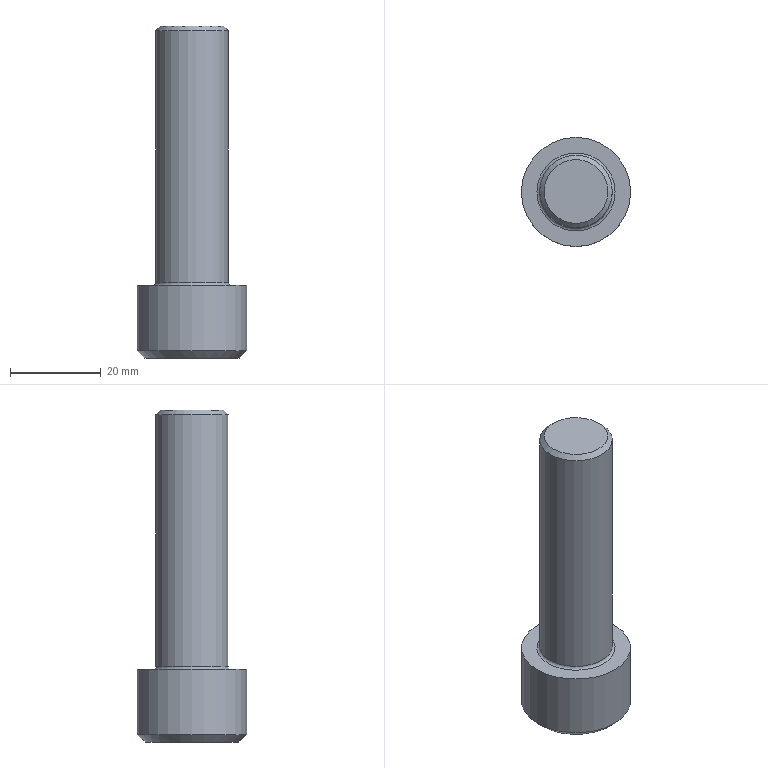Part | STEP file | solid 8 | 1 solid | 21 faces | box 24 x 24 x 73 mm | volume 17222 mm3 | plane 10 | sphere 6 | cylinder 2 | cone 2 | torus 1 | commonest cylinder face diameters 16 x1 24 x1